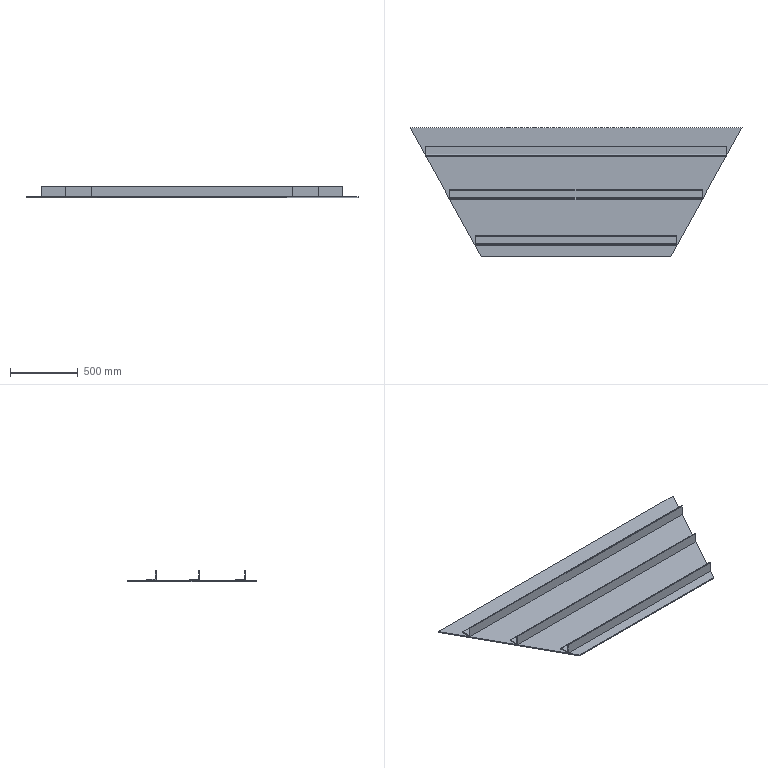Part | STEP file | Rear baffle assembly 2_Default<As machined> | 4 solids | 39 faces | box 2450 x 950 x 83 mm | volume 21025838 mm3 | plane 30 | cylinder 9 | commonest cylinder face diameters 5.333 x6 18 x3